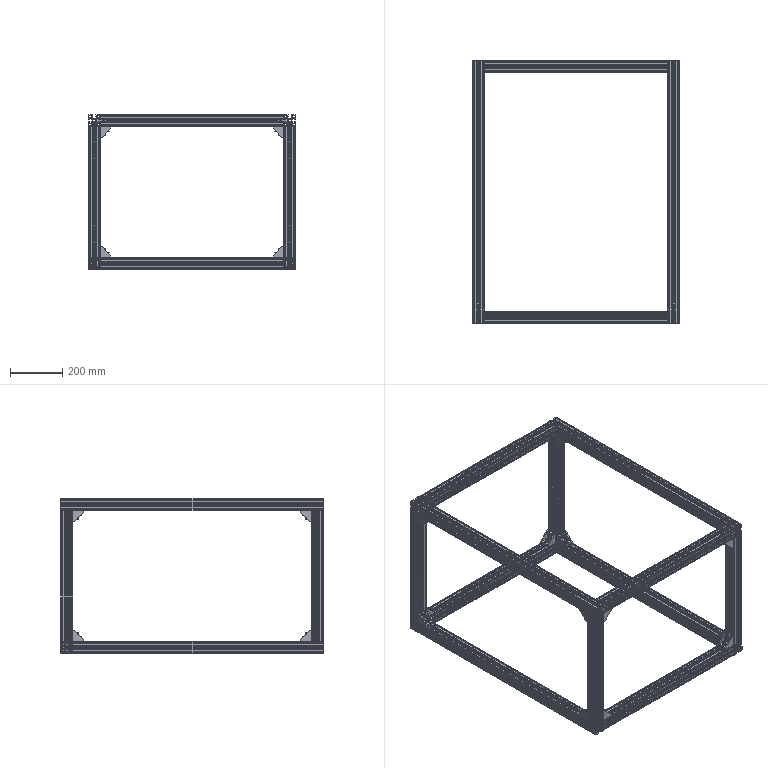Part | SolidWorks | 12 solids | 5834 faces | volume 5781926 mm3 | plane 4454 | cylinder 1192 | cone 132 | torus 56 | commonest cylinder face diameters 2 x432 10 x136 3 x120 12 x120 12.88 x84 6.8 x64